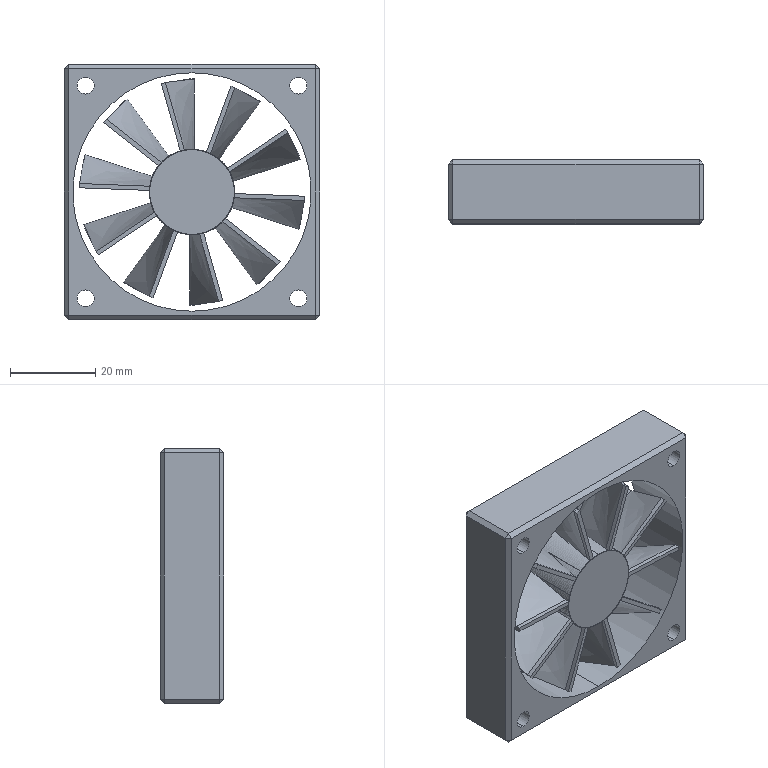Part | STEP file | Fan 60 | 11 solids | 176 faces | box 60 x 15 x 60 mm | volume 65760 mm3 | plane 106 | cylinder 40 | spline 30 | commonest cylinder face diameters 20 x30 4 x8 56 x2